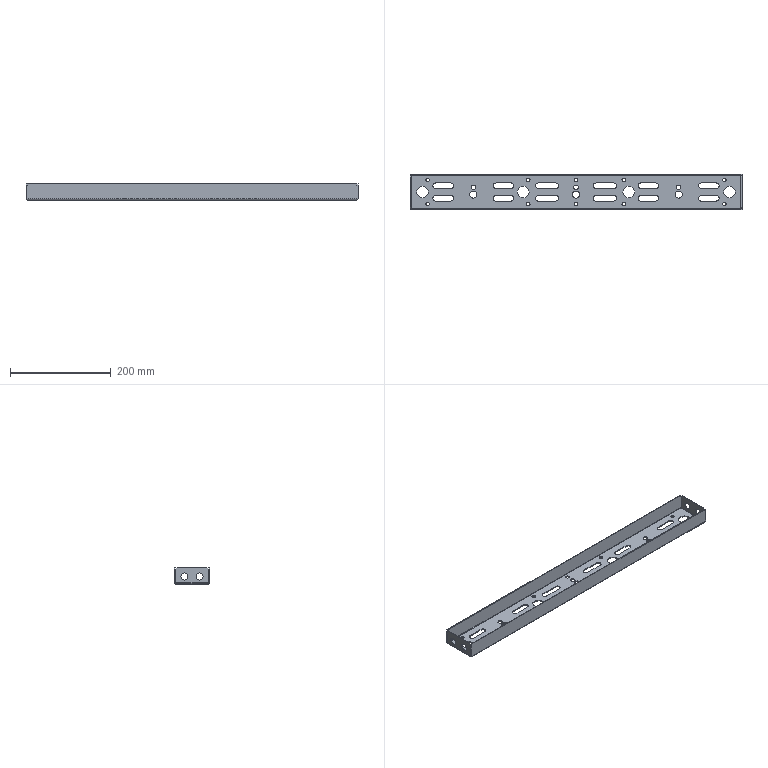Part | STEP file | Channel plate 2 | 1 solid | 158 faces | box 659.8 x 70 x 32 mm | volume 159810 mm3 | cylinder 92 | plane 58 | spline 8 | commonest cylinder face diameters 11 x36 7 x20 14 x14 23 x8 9 x6 1.473 x4